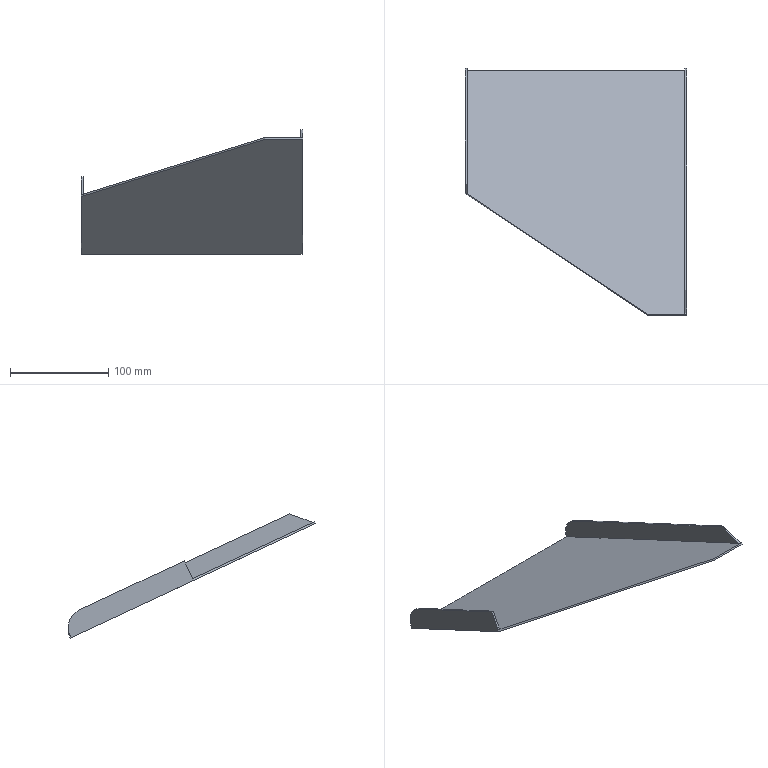Part | NX | features solid 2 | 1 solid | 15 faces | box 225.691 x 251.874 x 126.251 mm | volume 113364 mm3 | plane 13 | cylinder 2 | commonest cylinder face diameters 40 x2
STEP:
#1=CARTESIAN_POINT('',(530.986,470.,-185.082));
#2=VERTEX_POINT('',#1);
#3=CARTESIAN_POINT('',(344.309,594.452,-243.115));
#4=VERTEX_POINT('',#3);
#5=CARTESIAN_POINT('',(383.264,568.481,-231.004));
#6=DIRECTION('',(-0.8055,0.537,-0.2504));
#7=VECTOR('',#6,1000.);
#8=LINE('',#5,#7);
#9=EDGE_CURVE('',#2,#4,#8,.T.);
#10=ORIENTED_EDGE('',*,*,#9,.F.);
#11=CARTESIAN_POINT('',(530.986,470.845,-183.269));
#12=VERTEX_POINT('',#11);
#13=CARTESIAN_POINT('',(530.986,470.845,-183.269));
#14=DIRECTION('',(0.,-0.4226,-0.9063));
#15=VECTOR('',#14,1000.);
#16=LINE('',#13,#15);
#17=EDGE_CURVE('',#12,#2,#16,.T.);
#18=ORIENTED_EDGE('',*,*,#17,.F.);
#19=CARTESIAN_POINT('',(344.309,595.297,-241.302));
#20=VERTEX_POINT('',#19);
#21=CARTESIAN_POINT('',(383.264,569.326,-229.192));
#22=DIRECTION('',(-0.8055,0.537,-0.2504));
#23=VECTOR('',#22,1000.);
#24=LINE('',#21,#23);
#25=EDGE_CURVE('',#12,#20,#24,.T.);
#26=ORIENTED_EDGE('',*,*,#25,.T.);
#27=CARTESIAN_POINT('',(344.309,595.297,-241.302));
#28=DIRECTION('',(0.,-0.4226,-0.9063));
#29=VECTOR('',#28,1000.);
#30=LINE('',#27,#29);
#31=EDGE_CURVE('',#20,#4,#30,.T.);
#32=ORIENTED_EDGE('',*,*,#31,.T.);
#33=EDGE_LOOP('',(#10,#18,#26,#32));
#34=FACE_BOUND('',#33,.T.);
#35=CARTESIAN_POINT('',(383.264,569.326,-229.192));
#36=DIRECTION('',(-0.5925,-0.7301,0.3404));
#37=DIRECTION('',(0.7764,-0.6302,0.));
#38=AXIS2_PLACEMENT_3D('',#35,#36,#37);
#39=PLANE('',#38);
#40=ADVANCED_FACE('',(#34),#39,.T.);
#41=CARTESIAN_POINT('',(570.,470.,-185.082));
#42=VERTEX_POINT('',#41);
#43=CARTESIAN_POINT('',(570.,470.,-185.082));
#44=DIRECTION('',(-1.,0.,0.));
#45=VECTOR('',#44,1000.);
#46=LINE('',#43,#45);
#47=EDGE_CURVE('',#2,#42,#46,.F.);
#48=ORIENTED_EDGE('',*,*,#47,.T.);
#49=CARTESIAN_POINT('',(570.,470.845,-183.269));
#50=VERTEX_POINT('',#49);
#51=CARTESIAN_POINT('',(570.,470.845,-183.269));
#52=DIRECTION('',(0.,-0.4226,-0.9063));
#53=VECTOR('',#52,1000.);
#54=LINE('',#51,#53);
#55=EDGE_CURVE('',#50,#42,#54,.T.);
#56=ORIENTED_EDGE('',*,*,#55,.F.);
#57=CARTESIAN_POINT('',(570.,470.845,-183.269));
#58=DIRECTION('',(-1.,0.,0.));
#59=VECTOR('',#58,1000.);
#60=LINE('',#57,#59);
#61=EDGE_CURVE('',#12,#50,#60,.F.);
#62=ORIENTED_EDGE('',*,*,#61,.F.);
#63=ORIENTED_EDGE('',*,*,#17,.T.);
#64=EDGE_LOOP('',(#48,#56,#62,#63));
#65=FACE_BOUND('',#64,.T.);
#66=CARTESIAN_POINT('',(570.,470.845,-183.269));
#67=DIRECTION('',(0.,0.9063,-0.4226));
#68=DIRECTION('',(0.,0.4226,0.9063));
#69=AXIS2_PLACEMENT_3D('',#66,#67,#68);
#70=PLANE('',#69);
#71=ADVANCED_FACE('',(#65),#70,.F.);
#72=ORIENTED_EDGE('',*,*,#55,.T.);
#73=CARTESIAN_POINT('',(570.,720.,-301.659));
#74=VERTEX_POINT('',#73);
#75=CARTESIAN_POINT('',(570.,581.797,-237.214));
#76=DIRECTION('',(0.,-0.9063,0.4226));
#77=VECTOR('',#76,1000.);
#78=LINE('',#75,#77);
#79=EDGE_CURVE('',#74,#42,#78,.T.);
#80=ORIENTED_EDGE('',*,*,#79,.F.);
#81=CARTESIAN_POINT('',(570.,710.326,-275.08));
#82=VERTEX_POINT('',#81);
#83=CARTESIAN_POINT('',(570.,701.874,-293.206));
#84=DIRECTION('',(-1.,0.,0.));
#85=DIRECTION('',(0.,0.,1.));
#86=AXIS2_PLACEMENT_3D('',#83,#84,#85);
#87=CIRCLE('',#86,20.);
#88=EDGE_CURVE('',#74,#82,#87,.F.);
#89=ORIENTED_EDGE('',*,*,#88,.T.);
#90=CARTESIAN_POINT('',(570.,496.579,-175.408));
#91=VERTEX_POINT('',#90);
#92=CARTESIAN_POINT('',(570.,728.452,-283.533));
#93=DIRECTION('',(0.,-0.9063,0.4226));
#94=VECTOR('',#93,1000.);
#95=LINE('',#92,#94);
#96=EDGE_CURVE('',#82,#91,#95,.T.);
#97=ORIENTED_EDGE('',*,*,#96,.T.);
#98=CARTESIAN_POINT('',(570.,472.658,-184.114));
#99=VERTEX_POINT('',#98);
#100=CARTESIAN_POINT('',(570.,470.,-185.082));
#101=DIRECTION('',(0.,-0.9397,-0.342));
#102=VECTOR('',#101,1000.);
#103=LINE('',#100,#102);
#104=EDGE_CURVE('',#91,#99,#103,.T.);
#105=ORIENTED_EDGE('',*,*,#104,.T.);
#106=CARTESIAN_POINT('',(570.,582.643,-235.401));
#107=DIRECTION('',(0.,-0.9063,0.4226));
#108=VECTOR('',#107,1000.);
#109=LINE('',#106,#108);
#110=EDGE_CURVE('',#99,#50,#109,.T.);
#111=ORIENTED_EDGE('',*,*,#110,.T.);
#112=EDGE_LOOP('',(#72,#80,#89,#97,#105,#111));
#113=FACE_BOUND('',#112,.T.);
#114=CARTESIAN_POINT('',(570.,582.643,-235.401));
#115=DIRECTION('',(1.,0.,0.));
#116=DIRECTION('',(0.,0.,-1.));
#117=AXIS2_PLACEMENT_3D('',#114,#115,#116);
#118=PLANE('',#117);
#119=ADVANCED_FACE('',(#113),#118,.T.);
#120=CARTESIAN_POINT('',(568.,720.,-301.659));
#121=VERTEX_POINT('',#120);
#122=CARTESIAN_POINT('',(568.,720.,-299.452));
#123=VERTEX_POINT('',#122);
#124=CARTESIAN_POINT('',(568.,720.,-430.));
#125=DIRECTION('',(0.,0.,-1.));
#126=VECTOR('',#125,1000.);
#127=LINE('',#124,#126);
#128=EDGE_CURVE('',#121,#123,#127,.F.);
#129=ORIENTED_EDGE('',*,*,#128,.F.);
#130=CARTESIAN_POINT('',(344.309,720.,-301.659));
#131=VERTEX_POINT('',#130);
#132=CARTESIAN_POINT('',(570.,720.,-301.659));
#133=DIRECTION('',(-1.,0.,0.));
#134=VECTOR('',#133,1000.);
#135=LINE('',#132,#134);
#136=EDGE_CURVE('',#131,#121,#135,.F.);
#137=ORIENTED_EDGE('',*,*,#136,.F.);
#138=CARTESIAN_POINT('',(344.309,720.,-299.452));
#139=VERTEX_POINT('',#138);
#140=CARTESIAN_POINT('',(344.309,720.,-430.));
#141=DIRECTION('',(0.,0.,1.));
#142=VECTOR('',#141,1000.);
#143=LINE('',#140,#142);
#144=EDGE_CURVE('',#139,#131,#143,.F.);
#145=ORIENTED_EDGE('',*,*,#144,.F.);
#146=CARTESIAN_POINT('',(346.309,720.,-299.452));
#147=VERTEX_POINT('',#146);
#148=CARTESIAN_POINT('',(570.,720.,-299.452));
#149=DIRECTION('',(-1.,0.,0.));
#150=VECTOR('',#149,1000.);
#151=LINE('',#148,#150);
#152=EDGE_CURVE('',#139,#147,#151,.F.);
#153=ORIENTED_EDGE('',*,*,#152,.T.);
#154=CARTESIAN_POINT('',(570.,720.,-299.452));
#155=DIRECTION('',(-1.,0.,0.));
#156=VECTOR('',#155,1000.);
#157=LINE('',#154,#156);
#158=EDGE_CURVE('',#147,#123,#157,.F.);
#159=ORIENTED_EDGE('',*,*,#158,.T.);
#160=EDGE_LOOP('',(#129,#137,#145,#153,#159));
#161=FACE_BOUND('',#160,.T.);
#162=CARTESIAN_POINT('',(188.564,720.,-430.));
#163=DIRECTION('',(0.,-1.,0.));
#164=DIRECTION('',(-1.,0.,0.));
#165=AXIS2_PLACEMENT_3D('',#162,#163,#164);
#166=PLANE('',#165);
#167=ADVANCED_FACE('',(#161),#166,.F.);
#168=CARTESIAN_POINT('',(344.309,524.315,-210.409));
#169=DIRECTION('',(0.,-0.9063,0.4226));
#170=VECTOR('',#169,1000.);
#171=LINE('',#168,#170);
#172=EDGE_CURVE('',#131,#4,#171,.T.);
#173=ORIENTED_EDGE('',*,*,#172,.T.);
#174=ORIENTED_EDGE('',*,*,#31,.F.);
#175=CARTESIAN_POINT('',(344.309,603.749,-223.176));
#176=VERTEX_POINT('',#175);
#177=CARTESIAN_POINT('',(344.309,595.297,-241.302));
#178=DIRECTION('',(0.,0.4226,0.9063));
#179=VECTOR('',#178,1000.);
#180=LINE('',#177,#179);
#181=EDGE_CURVE('',#20,#176,#180,.T.);
#182=ORIENTED_EDGE('',*,*,#181,.T.);
#183=CARTESIAN_POINT('',(344.309,710.326,-272.873));
#184=VERTEX_POINT('',#183);
#185=CARTESIAN_POINT('',(344.309,728.452,-281.326));
#186=DIRECTION('',(0.,-0.9063,0.4226));
#187=VECTOR('',#186,1000.);
#188=LINE('',#185,#187);
#189=EDGE_CURVE('',#184,#176,#188,.T.);
#190=ORIENTED_EDGE('',*,*,#189,.F.);
#191=CARTESIAN_POINT('',(344.309,701.874,-291.));
#192=DIRECTION('',(-1.,0.,0.));
#193=DIRECTION('',(0.,-1.,0.));
#194=AXIS2_PLACEMENT_3D('',#191,#192,#193);
#195=CIRCLE('',#194,20.);
#196=EDGE_CURVE('',#184,#139,#195,.T.);
#197=ORIENTED_EDGE('',*,*,#196,.T.);
#198=ORIENTED_EDGE('',*,*,#144,.T.);
#199=EDGE_LOOP('',(#173,#174,#182,#190,#197,#198));
#200=FACE_BOUND('',#199,.T.);
#201=CARTESIAN_POINT('',(344.309,525.16,-208.597));
#202=DIRECTION('',(1.,0.,0.));
#203=DIRECTION('',(0.,1.,0.));
#204=AXIS2_PLACEMENT_3D('',#201,#202,#203);
#205=PLANE('',#204);
#206=ADVANCED_FACE('',(#200),#205,.F.);
#207=CARTESIAN_POINT('',(568.,472.658,-184.114));
#208=VERTEX_POINT('',#207);
#209=CARTESIAN_POINT('',(570.,472.658,-184.114));
#210=DIRECTION('',(-1.,0.,0.));
#211=VECTOR('',#210,1000.);
#212=LINE('',#209,#211);
#213=EDGE_CURVE('',#99,#208,#212,.T.);
#214=ORIENTED_EDGE('',*,*,#213,.T.);
#215=CARTESIAN_POINT('',(568.,582.643,-235.401));
#216=DIRECTION('',(0.,0.9063,-0.4226));
#217=VECTOR('',#216,1000.);
#218=LINE('',#215,#217);
#219=EDGE_CURVE('',#208,#123,#218,.T.);
#220=ORIENTED_EDGE('',*,*,#219,.T.);
#221=ORIENTED_EDGE('',*,*,#158,.F.);
#222=CARTESIAN_POINT('',(346.309,595.297,-241.302));
#223=VERTEX_POINT('',#222);
#224=CARTESIAN_POINT('',(346.309,720.,-299.452));
#225=DIRECTION('',(0.,-0.9063,0.4226));
#226=VECTOR('',#225,1000.);
#227=LINE('',#224,#226);
#228=EDGE_CURVE('',#147,#223,#227,.T.);
#229=ORIENTED_EDGE('',*,*,#228,.T.);
#230=CARTESIAN_POINT('',(344.309,595.297,-241.302));
#231=DIRECTION('',(1.,0.,0.));
#232=VECTOR('',#231,1000.);
#233=LINE('',#230,#232);
#234=EDGE_CURVE('',#20,#223,#233,.T.);
#235=ORIENTED_EDGE('',*,*,#234,.F.);
#236=ORIENTED_EDGE('',*,*,#25,.F.);
#237=ORIENTED_EDGE('',*,*,#61,.T.);
#238=ORIENTED_EDGE('',*,*,#110,.F.);
#239=EDGE_LOOP('',(#214,#220,#221,#229,#235,#236,#237,#238));
#240=FACE_BOUND('',#239,.T.);
#241=CARTESIAN_POINT('',(570.,582.643,-235.401));
#242=DIRECTION('',(0.,-0.4226,-0.9063));
#243=DIRECTION('',(-1.,0.,0.));
#244=AXIS2_PLACEMENT_3D('',#241,#242,#243);
#245=PLANE('',#244);
#246=ADVANCED_FACE('',(#240),#245,.F.);
#247=ORIENTED_EDGE('',*,*,#136,.T.);
#248=CARTESIAN_POINT('',(570.,720.,-301.659));
#249=DIRECTION('',(1.,0.,0.));
#250=VECTOR('',#249,1000.);
#251=LINE('',#248,#250);
#252=EDGE_CURVE('',#74,#121,#251,.F.);
#253=ORIENTED_EDGE('',*,*,#252,.F.);
#254=ORIENTED_EDGE('',*,*,#79,.T.);
#255=ORIENTED_EDGE('',*,*,#47,.F.);
#256=ORIENTED_EDGE('',*,*,#9,.T.);
#257=ORIENTED_EDGE('',*,*,#172,.F.);
#258=EDGE_LOOP('',(#247,#253,#254,#255,#256,#257));
#259=FACE_BOUND('',#258,.T.);
#260=CARTESIAN_POINT('',(570.,581.797,-237.214));
#261=DIRECTION('',(0.,-0.4226,-0.9063));
#262=DIRECTION('',(-1.,0.,0.));
#263=AXIS2_PLACEMENT_3D('',#260,#261,#262);
#264=PLANE('',#263);
#265=ADVANCED_FACE('',(#259),#264,.T.);
#266=CARTESIAN_POINT('',(346.309,710.326,-272.873));
#267=VERTEX_POINT('',#266);
#268=CARTESIAN_POINT('',(346.309,603.749,-223.176));
#269=VERTEX_POINT('',#268);
#270=CARTESIAN_POINT('',(346.309,728.452,-281.326));
#271=DIRECTION('',(0.,-0.9063,0.4226));
#272=VECTOR('',#271,1000.);
#273=LINE('',#270,#272);
#274=EDGE_CURVE('',#267,#269,#273,.T.);
#275=ORIENTED_EDGE('',*,*,#274,.F.);
#276=CARTESIAN_POINT('',(344.309,710.326,-272.873));
#277=DIRECTION('',(-1.,0.,0.));
#278=VECTOR('',#277,1000.);
#279=LINE('',#276,#278);
#280=EDGE_CURVE('',#267,#184,#279,.T.);
#281=ORIENTED_EDGE('',*,*,#280,.T.);
#282=ORIENTED_EDGE('',*,*,#189,.T.);
#283=CARTESIAN_POINT('',(344.309,603.749,-223.176));
#284=DIRECTION('',(1.,0.,0.));
#285=VECTOR('',#284,1000.);
#286=LINE('',#283,#285);
#287=EDGE_CURVE('',#176,#269,#286,.T.);
#288=ORIENTED_EDGE('',*,*,#287,.T.);
#289=EDGE_LOOP('',(#275,#281,#282,#288));
#290=FACE_BOUND('',#289,.T.);
#291=CARTESIAN_POINT('',(344.309,728.452,-281.326));
#292=DIRECTION('',(0.,-0.4226,-0.9063));
#293=DIRECTION('',(0.,-0.9063,0.4226));
#294=AXIS2_PLACEMENT_3D('',#291,#292,#293);
#295=PLANE('',#294);
#296=ADVANCED_FACE('',(#290),#295,.F.);
#297=ORIENTED_EDGE('',*,*,#228,.F.);
#298=CARTESIAN_POINT('',(346.309,701.874,-291.));
#299=DIRECTION('',(-1.,0.,0.));
#300=DIRECTION('',(0.,-1.,0.));
#301=AXIS2_PLACEMENT_3D('',#298,#299,#300);
#302=CIRCLE('',#301,20.);
#303=EDGE_CURVE('',#147,#267,#302,.F.);
#304=ORIENTED_EDGE('',*,*,#303,.T.);
#305=ORIENTED_EDGE('',*,*,#274,.T.);
#306=CARTESIAN_POINT('',(346.309,595.297,-241.302));
#307=DIRECTION('',(0.,0.4226,0.9063));
#308=VECTOR('',#307,1000.);
#309=LINE('',#306,#308);
#310=EDGE_CURVE('',#223,#269,#309,.T.);
#311=ORIENTED_EDGE('',*,*,#310,.F.);
#312=EDGE_LOOP('',(#297,#304,#305,#311));
#313=FACE_BOUND('',#312,.T.);
#314=CARTESIAN_POINT('',(346.309,720.,-299.452));
#315=DIRECTION('',(-1.,0.,0.));
#316=DIRECTION('',(0.,-1.,0.));
#317=AXIS2_PLACEMENT_3D('',#314,#315,#316);
#318=PLANE('',#317);
#319=ADVANCED_FACE('',(#313),#318,.F.);
#320=ORIENTED_EDGE('',*,*,#181,.F.);
#321=ORIENTED_EDGE('',*,*,#234,.T.);
#322=ORIENTED_EDGE('',*,*,#310,.T.);
#323=ORIENTED_EDGE('',*,*,#287,.F.);
#324=EDGE_LOOP('',(#320,#321,#322,#323));
#325=FACE_BOUND('',#324,.T.);
#326=CARTESIAN_POINT('',(344.309,595.297,-241.302));
#327=DIRECTION('',(0.,-0.9063,0.4226));
#328=DIRECTION('',(0.,0.4226,0.9063));
#329=AXIS2_PLACEMENT_3D('',#326,#327,#328);
#330=PLANE('',#329);
#331=ADVANCED_FACE('',(#325),#330,.T.);
#332=ORIENTED_EDGE('',*,*,#196,.F.);
#333=ORIENTED_EDGE('',*,*,#280,.F.);
#334=ORIENTED_EDGE('',*,*,#303,.F.);
#335=ORIENTED_EDGE('',*,*,#152,.F.);
#336=EDGE_LOOP('',(#332,#333,#334,#335));
#337=FACE_BOUND('',#336,.T.);
#338=CARTESIAN_POINT('',(344.309,701.874,-291.));
#339=DIRECTION('',(1.,0.,0.));
#340=DIRECTION('',(0.,1.,0.));
#341=AXIS2_PLACEMENT_3D('',#338,#339,#340);
#342=CYLINDRICAL_SURFACE('',#341,20.);
#343=ADVANCED_FACE('',(#337),#342,.T.);
#344=ORIENTED_EDGE('',*,*,#213,.F.);
#345=ORIENTED_EDGE('',*,*,#104,.F.);
#346=CARTESIAN_POINT('',(568.,496.579,-175.408));
#347=VERTEX_POINT('',#346);
#348=CARTESIAN_POINT('',(570.,496.579,-175.408));
#349=DIRECTION('',(1.,0.,0.));
#350=VECTOR('',#349,1000.);
#351=LINE('',#348,#350);
#352=EDGE_CURVE('',#347,#91,#351,.T.);
#353=ORIENTED_EDGE('',*,*,#352,.F.);
#354=CARTESIAN_POINT('',(568.,653.288,-118.37));
#355=DIRECTION('',(0.,0.9397,0.342));
#356=VECTOR('',#355,1000.);
#357=LINE('',#354,#356);
#358=EDGE_CURVE('',#208,#347,#357,.T.);
#359=ORIENTED_EDGE('',*,*,#358,.F.);
#360=EDGE_LOOP('',(#344,#345,#353,#359));
#361=FACE_BOUND('',#360,.T.);
#362=CARTESIAN_POINT('',(570.,470.,-185.082));
#363=DIRECTION('',(0.,-0.342,0.9397));
#364=DIRECTION('',(0.,-0.9397,-0.342));
#365=AXIS2_PLACEMENT_3D('',#362,#363,#364);
#366=PLANE('',#365);
#367=ADVANCED_FACE('',(#361),#366,.T.);
#368=ORIENTED_EDGE('',*,*,#96,.F.);
#369=CARTESIAN_POINT('',(568.,710.326,-275.08));
#370=VERTEX_POINT('',#369);
#371=CARTESIAN_POINT('',(570.,710.326,-275.08));
#372=DIRECTION('',(-1.,0.,0.));
#373=VECTOR('',#372,1000.);
#374=LINE('',#371,#373);
#375=EDGE_CURVE('',#82,#370,#374,.T.);
#376=ORIENTED_EDGE('',*,*,#375,.T.);
#377=CARTESIAN_POINT('',(568.,728.452,-283.533));
#378=DIRECTION('',(0.,-0.9063,0.4226));
#379=VECTOR('',#378,1000.);
#380=LINE('',#377,#379);
#381=EDGE_CURVE('',#370,#347,#380,.T.);
#382=ORIENTED_EDGE('',*,*,#381,.T.);
#383=ORIENTED_EDGE('',*,*,#352,.T.);
#384=EDGE_LOOP('',(#368,#376,#382,#383));
#385=FACE_BOUND('',#384,.T.);
#386=CARTESIAN_POINT('',(570.,728.452,-283.533));
#387=DIRECTION('',(0.,-0.4226,-0.9063));
#388=DIRECTION('',(0.,-0.9063,0.4226));
#389=AXIS2_PLACEMENT_3D('',#386,#387,#388);
#390=PLANE('',#389);
#391=ADVANCED_FACE('',(#385),#390,.F.);
#392=CARTESIAN_POINT('',(568.,701.874,-293.206));
#393=DIRECTION('',(-1.,0.,0.));
#394=DIRECTION('',(0.,0.,1.));
#395=AXIS2_PLACEMENT_3D('',#392,#393,#394);
#396=CIRCLE('',#395,20.);
#397=EDGE_CURVE('',#370,#121,#396,.T.);
#398=ORIENTED_EDGE('',*,*,#397,.T.);
#399=ORIENTED_EDGE('',*,*,#128,.T.);
#400=ORIENTED_EDGE('',*,*,#219,.F.);
#401=ORIENTED_EDGE('',*,*,#358,.T.);
#402=ORIENTED_EDGE('',*,*,#381,.F.);
#403=EDGE_LOOP('',(#398,#399,#400,#401,#402));
#404=FACE_BOUND('',#403,.T.);
#405=CARTESIAN_POINT('',(568.,720.,-301.659));
#406=DIRECTION('',(-1.,0.,0.));
#407=DIRECTION('',(0.,0.,1.));
#408=AXIS2_PLACEMENT_3D('',#405,#406,#407);
#409=PLANE('',#408);
#410=ADVANCED_FACE('',(#404),#409,.T.);
#411=ORIENTED_EDGE('',*,*,#88,.F.);
#412=ORIENTED_EDGE('',*,*,#252,.T.);
#413=ORIENTED_EDGE('',*,*,#397,.F.);
#414=ORIENTED_EDGE('',*,*,#375,.F.);
#415=EDGE_LOOP('',(#411,#412,#413,#414));
#416=FACE_BOUND('',#415,.T.);
#417=CARTESIAN_POINT('',(570.,701.874,-293.206));
#418=DIRECTION('',(-1.,0.,0.));
#419=DIRECTION('',(0.,0.,1.));
#420=AXIS2_PLACEMENT_3D('',#417,#418,#419);
#421=CYLINDRICAL_SURFACE('',#420,20.);
#422=ADVANCED_FACE('',(#416),#421,.T.);
#423=CLOSED_SHELL('',(#40,#71,#119,#167,#206,#246,#265,#296,#319,#331,#343,#367,#391,#410,#422));
#424=MANIFOLD_SOLID_BREP('',#423);
#425=(LENGTH_UNIT()NAMED_UNIT(*)SI_UNIT(.MILLI.,.METRE.));
#426=UNCERTAINTY_MEASURE_WITH_UNIT(LENGTH_MEASURE(0.00001),#425,'','');
#427=(NAMED_UNIT(*)PLANE_ANGLE_UNIT()SI_UNIT($,.RADIAN.));
#428=(NAMED_UNIT(*)SI_UNIT($,.STERADIAN.)SOLID_ANGLE_UNIT());
#429=(GEOMETRIC_REPRESENTATION_CONTEXT(3)GLOBAL_UNCERTAINTY_ASSIGNED_CONTEXT((#426))GLOBAL_UNIT_ASSIGNED_CONTEXT((#425,#427,#428))REPRESENTATION_CONTEXT('',''));
#430=ADVANCED_BREP_SHAPE_REPRESENTATION('',(#424),#429);